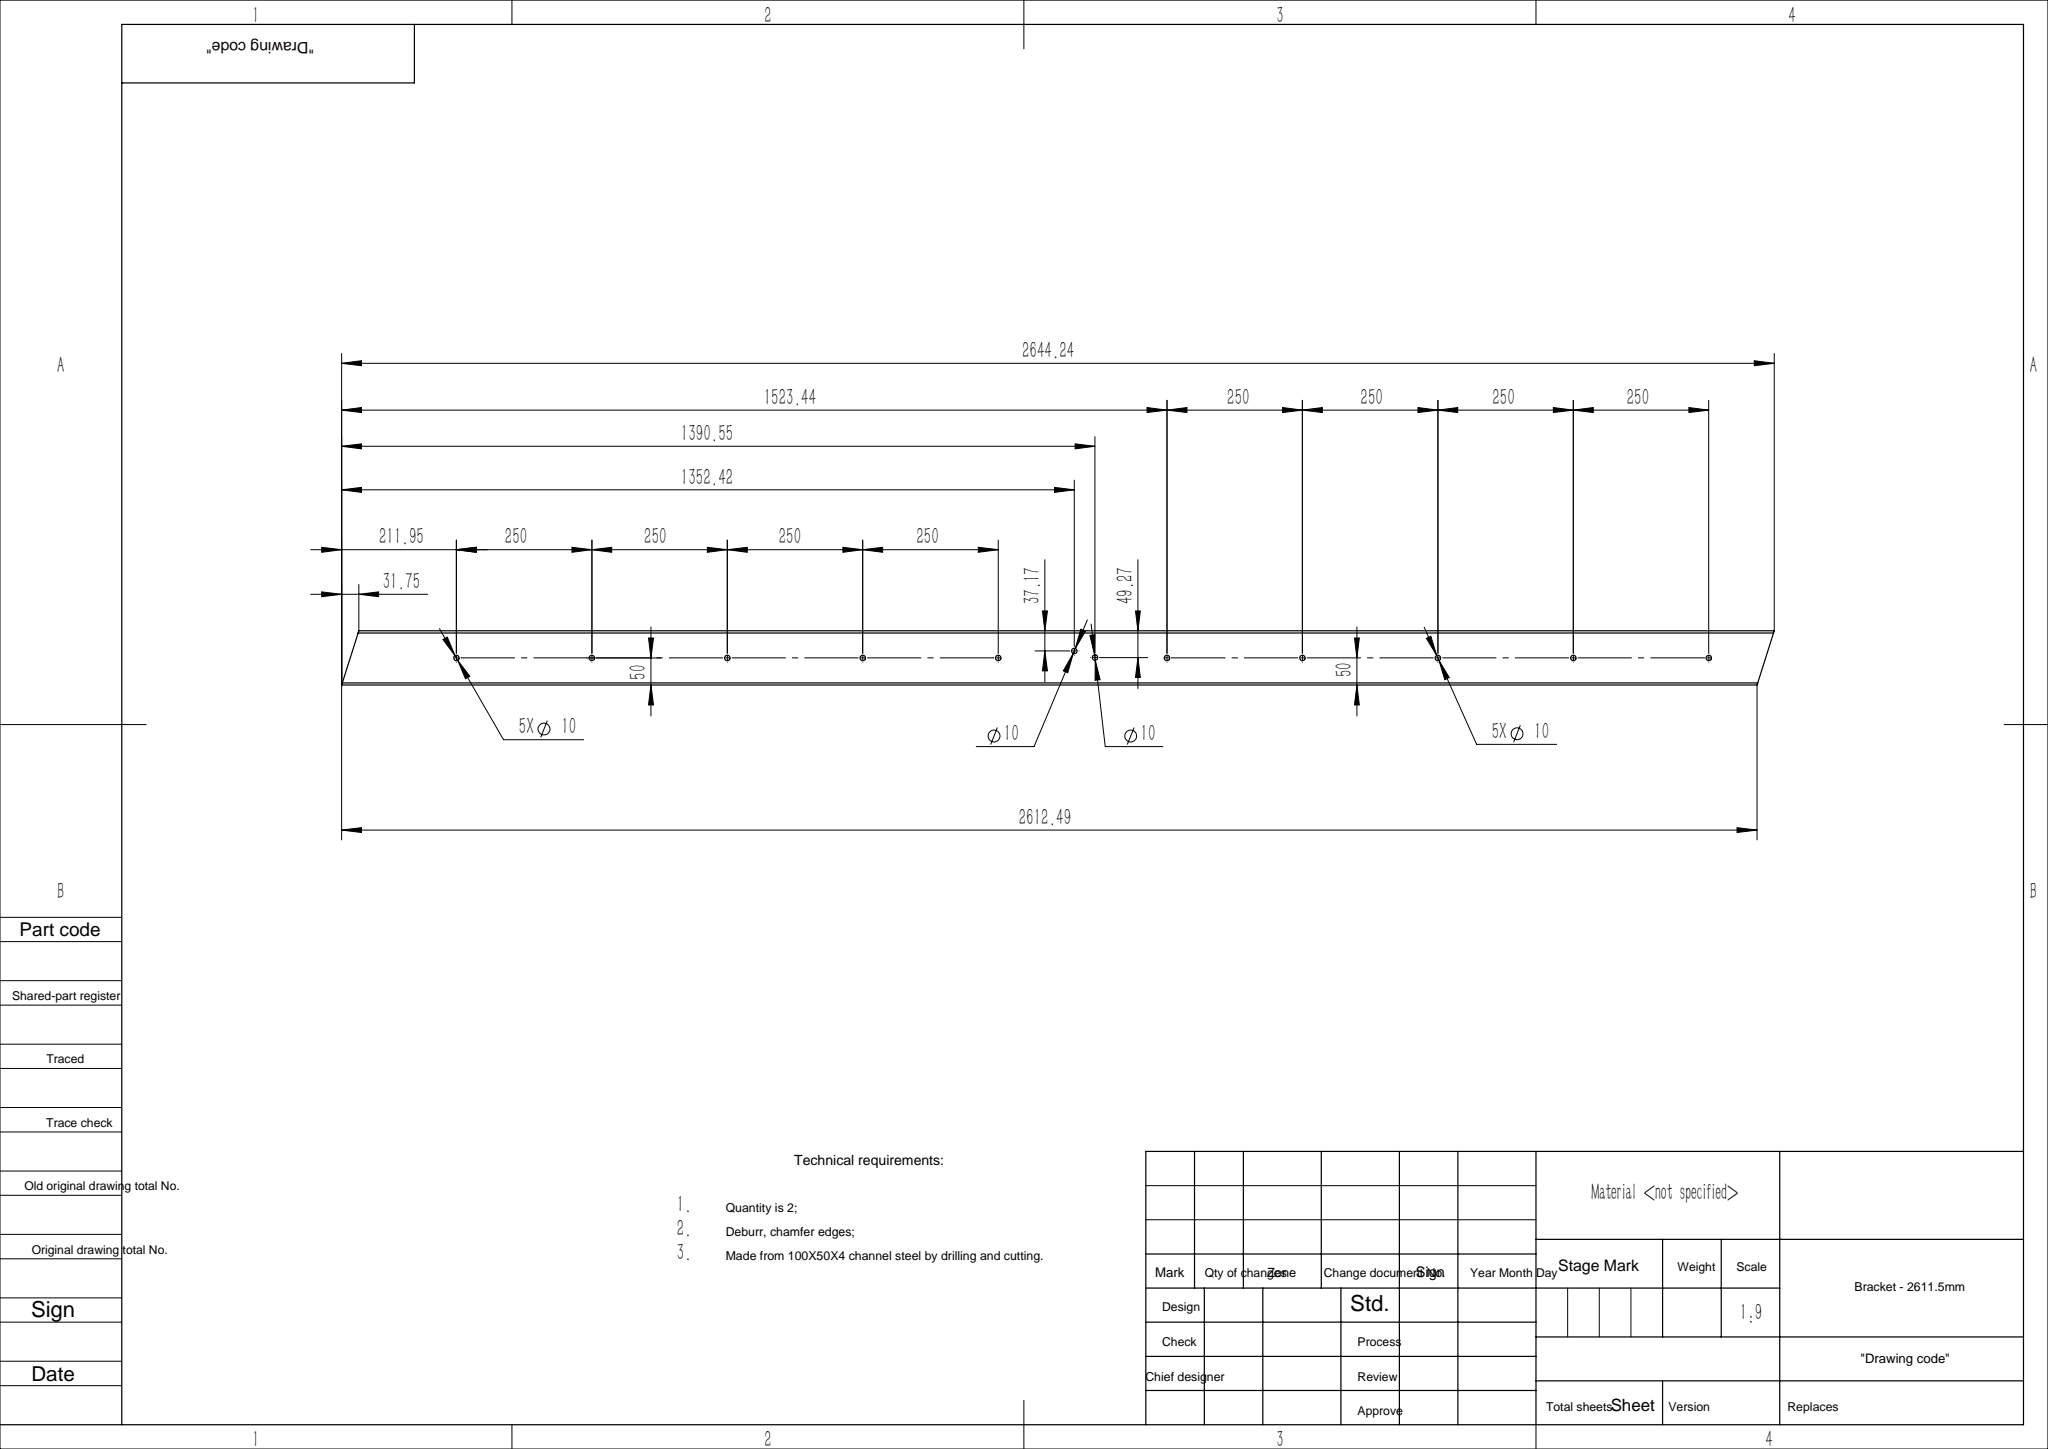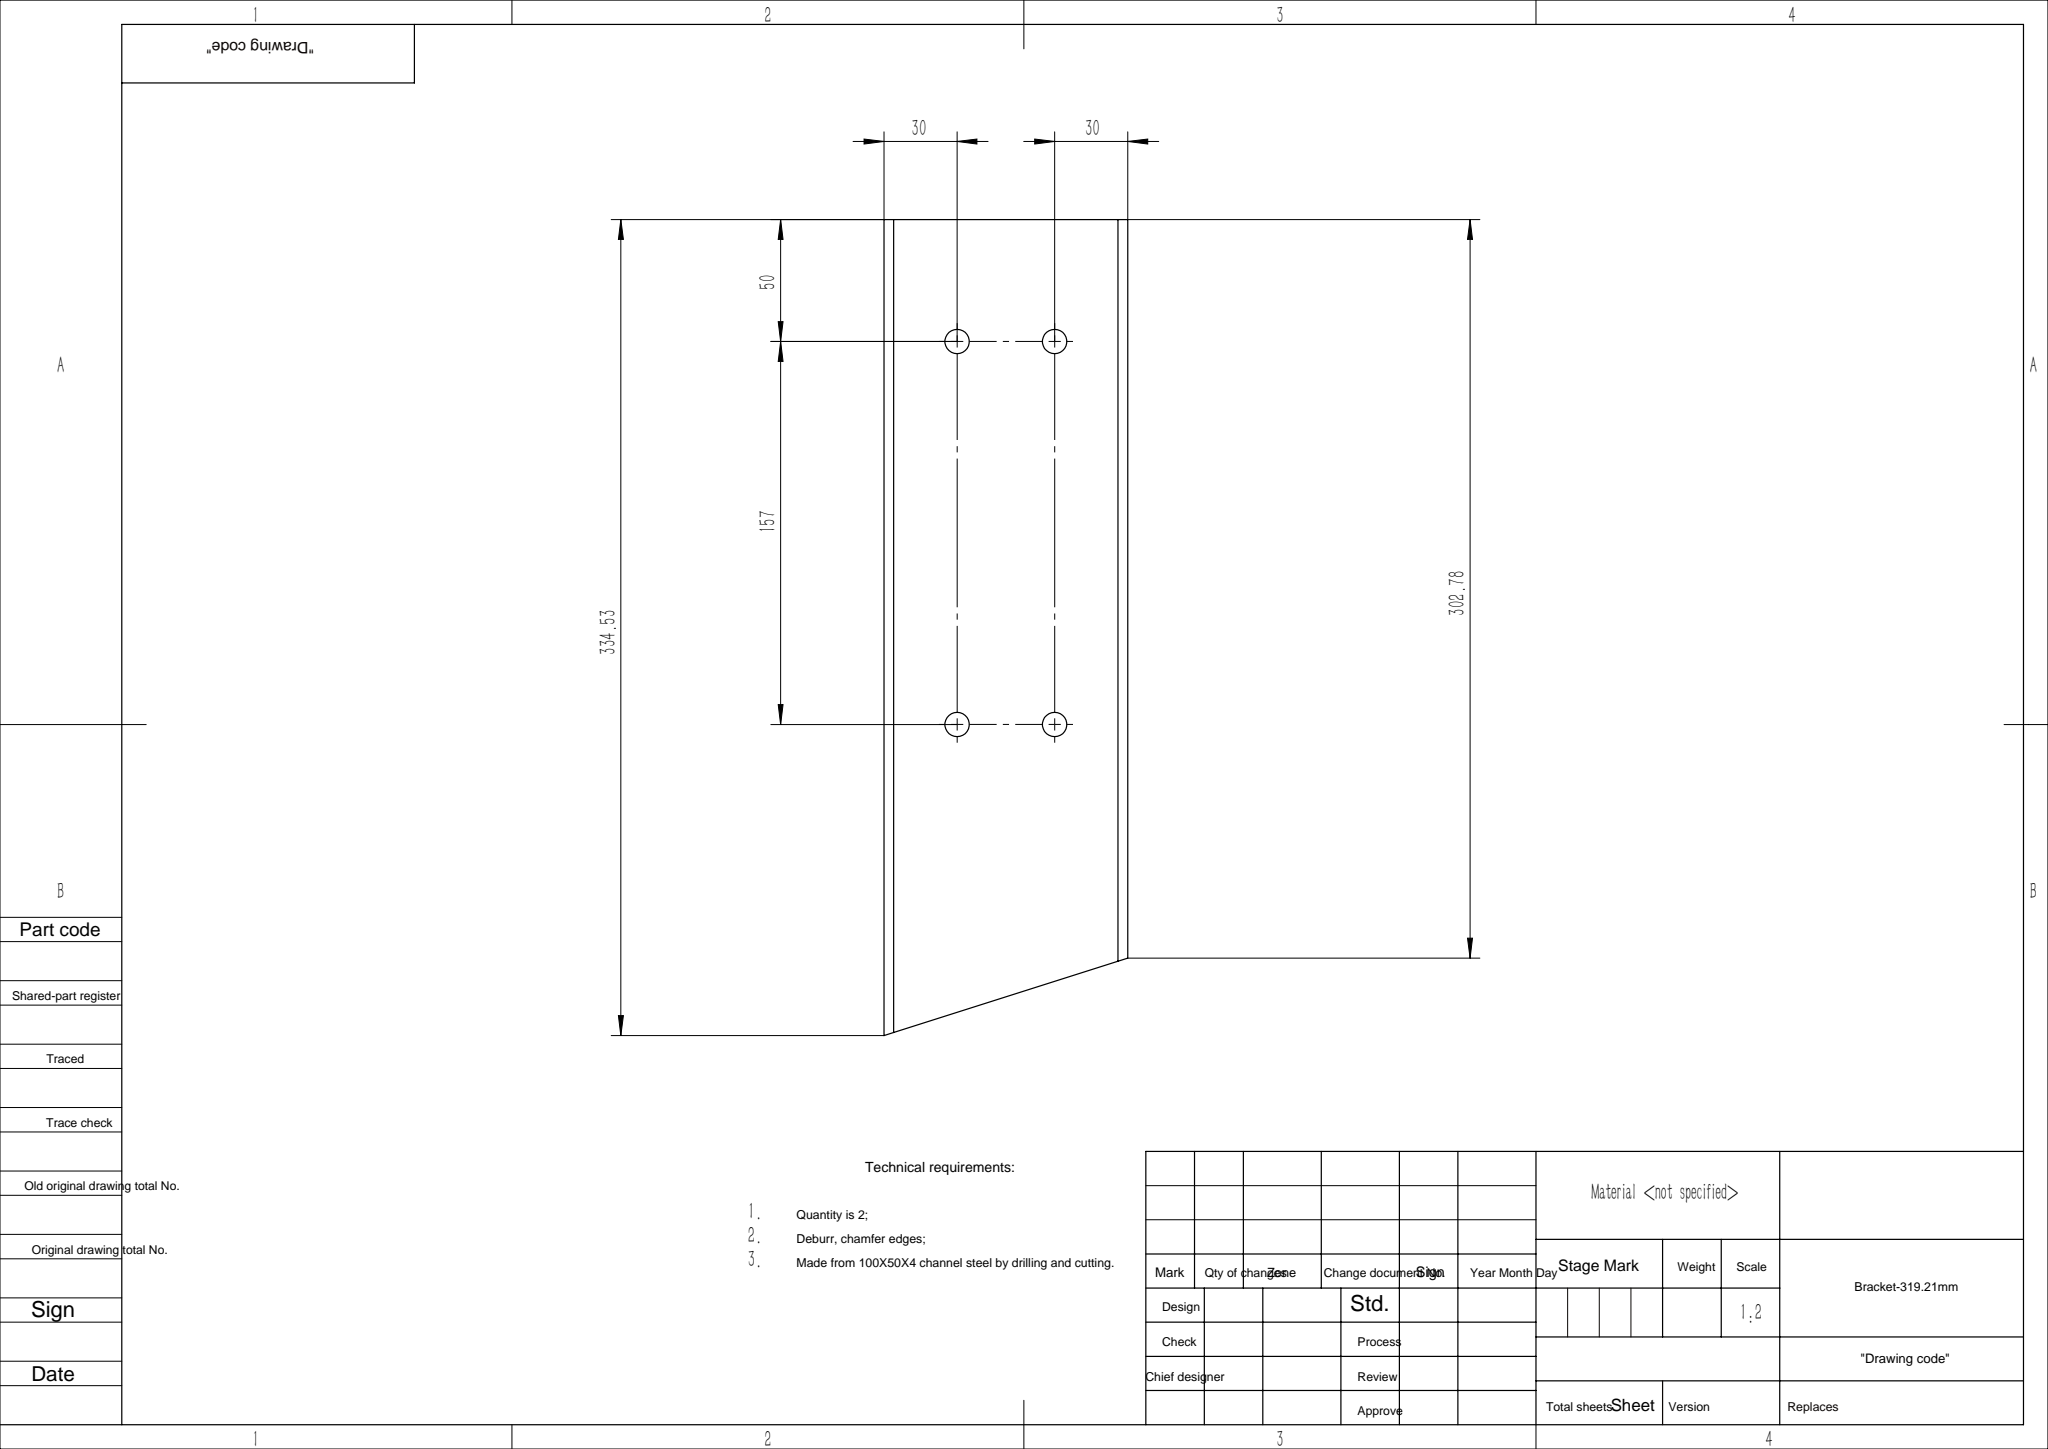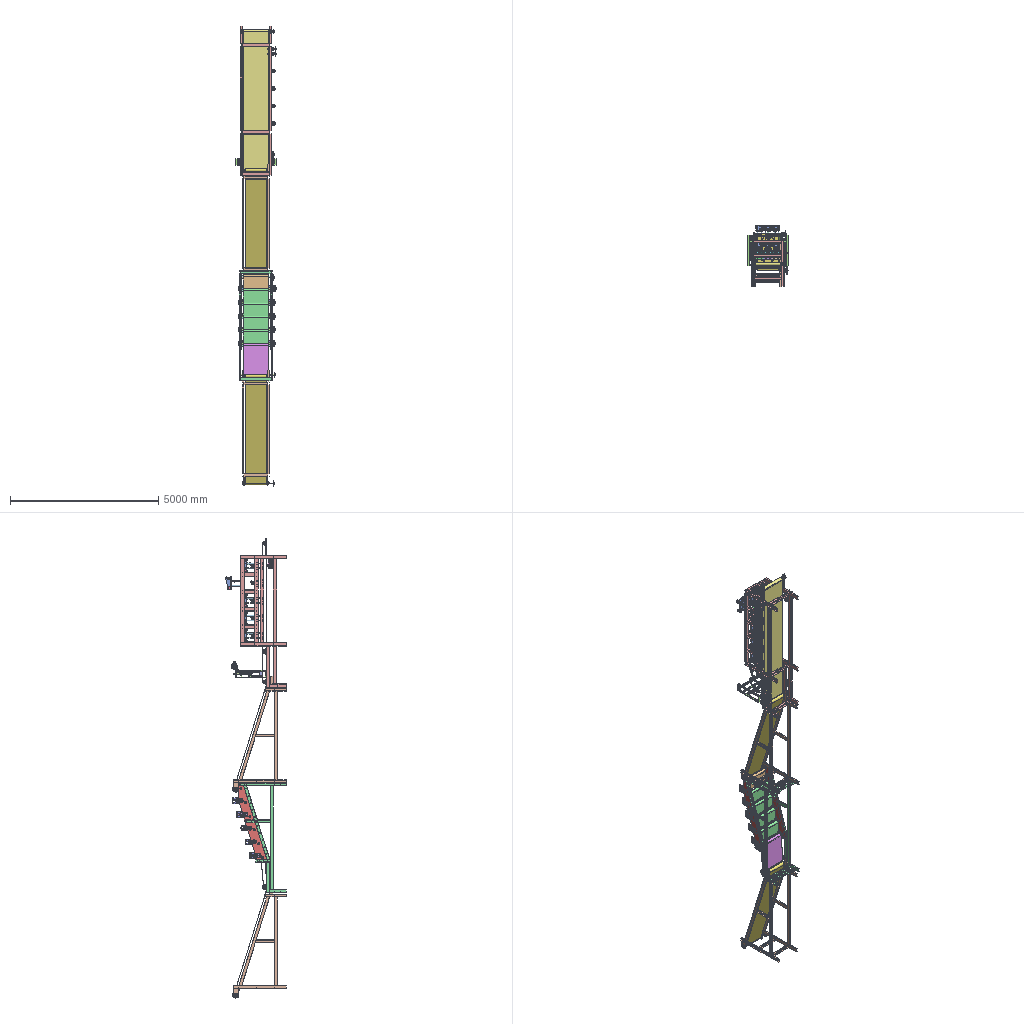Assembly | SolidWorks | 119 different items | 1543 placed | box 1379 x 2047 x 15524 mm
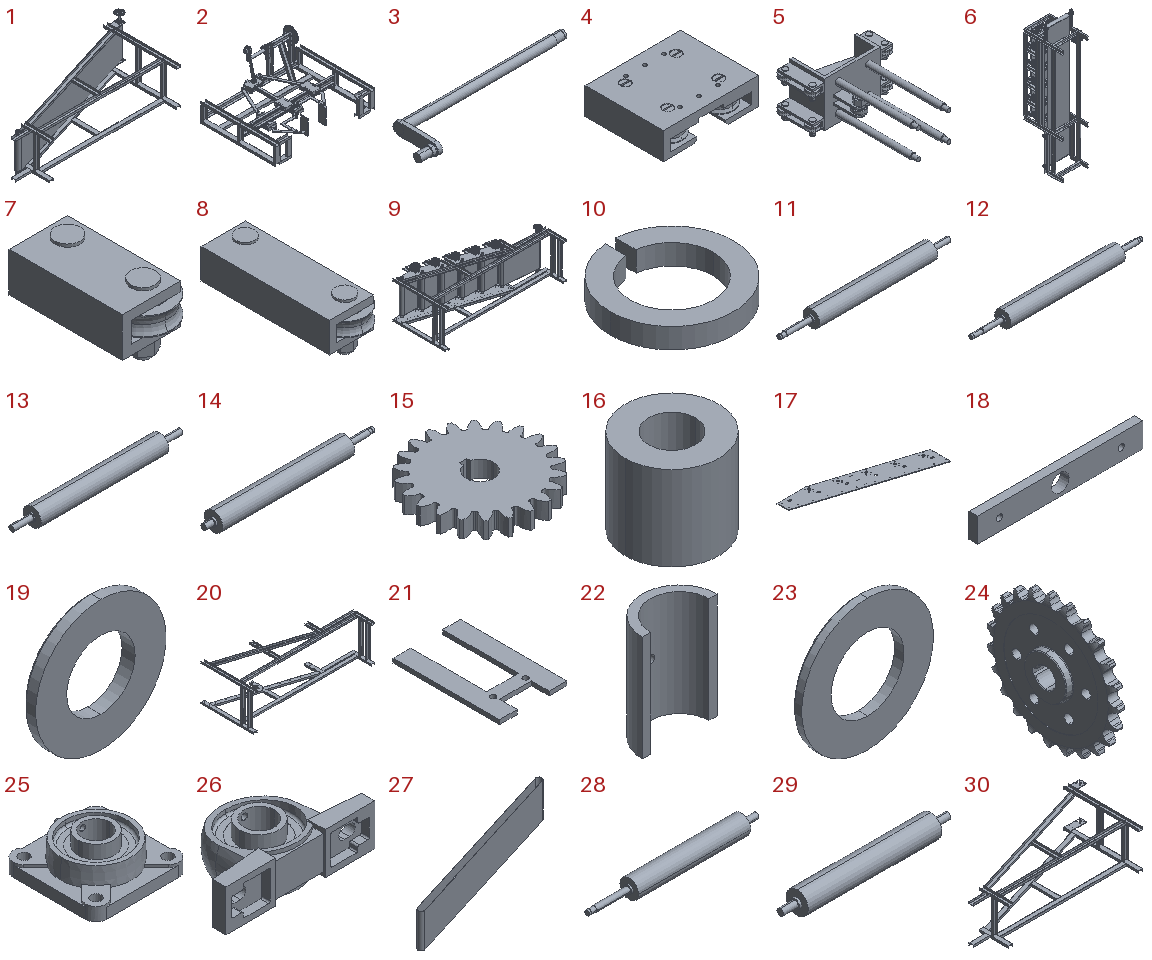Parts list (item | name | quantity | parent item | size | volume | features):
1 | (subassembly) | x2 | - | 3909 x 1808 x 1083 mm | 53217472 mm3 | features MirrorCompFeat 2, ReferencePattern 2
2 | (subassembly) | x1 | - | - | 12242540 mm3 | features LocalLPattern 2, ReferencePattern 2
3 | (subassembly) | x1 | in 2 | 687.7 x 174.987 x 46.865 mm | 737017 mm3 | -
4 | (subassembly) | x5 | in 2 | 135 x 110 x 38 mm | 364943 mm3 | features ReferencePattern 15, LocalLPattern 1
5 | (subassembly) | x15 | in 6 | 430 x 604 x 239 mm | 5255381 mm3 | features ReferencePattern 10, CompositeCurve 1, LocalSketchPattern 1, MirrorCompFeat 1
6 | (subassembly) | x1 | - | - | 264532636 mm3 | features ReferencePattern 140, InContextFeatHolder 10, LocalLPattern 2, LocalSketchPattern 2, MirrorCompFeat 2
7 | (subassembly) | x30 | in 5 | 72 x 140 x 70 mm | 285361 mm3 | -
8 | (subassembly) | x30 | in 5 | 72 x 200 x 70 mm | 372961 mm3 | -
9 | (subassembly) | x1 | - | - | 262282072 mm3 | features ReferencePattern 142, LocalLPattern 5, CompositeCurve 3, MirrorCompFeat 3, AEMSimFeature 1, LocalSketchPattern 1
10 | - | x1 | in 2 | 45.424 x 45.346 x 7.5 mm | 6464 mm3 | features Extrusion 1
11 | - | x1 | in 9 | 1221 x 120 x 120 mm | 9978087 mm3 | features ICE 2, Revolution 1
12 | - | x5 | in 9 | 1261 x 120 x 120 mm | 9997554 mm3 | features ICE 4, Revolution 1
13 | - | x6 | in 9 | 1122 x 120 x 120 mm | 9905091 mm3 | features 3DProfileFeature 1, HoleWzd 1, MirrorPattern 1, Revolution 1
14 | - | x5 | in 9 | 1088 x 120 x 120 mm | 9853270 mm3 | features ICE 2, Revolution 1
15 | - | x10 | in 9 | 133.882 x 132.987 x 18 mm | 197482 mm3 | features ICE 2, CirPattern 1, Extrusion 1, RefAxis 1
16 | - | x20 | in 9 | 30 x 30 x 27 mm | 14314 mm3 | features Extrusion 1
17 | - | x2 | in 9 | 2640 x 1075 x 12 mm | 12600247 mm3 | features Cut 7, LPattern 5, ICE 2, Extrusion 1, SurfCut 1
18 | - | x10 | in 9 | 190 x 10 x 28 mm | 49289 mm3 | features Cut 1, Extrusion 1
19 | - | x1 | in 2 | 20 x 2 x 20 mm | 447.415 mm3 | features Revolution 1
20 | - | x1 | in 9 | 3700 x 1611 x 1120 mm | 19309543 mm3 | features ICE 8, Cut 6, LPattern 6, Extrusion 1, MirrorPattern 1
21 | - | x10 | in 9 | 190 x 300 x 12 mm | 394178 mm3 | features Extrusion 1, HoleWzd 1
22 | - | x12 | in 9 | 46 x 23 x 65 mm | 20833 mm3 | features 3DProfileFeature 1, Extrusion 1, HoleWzd 1
23 | - | x1 | in 2 | 56 x 4 x 56 mm | 6746 mm3 | features Revolution 1
24 | - | x12 | in 9 | 32 x 197.271 x 197.721 mm | 369448 mm3 | features Cut 3, CirPattern 2, Revolution 2, Chamfer 1, Fillet 1, MirrorPattern 1
25 | - | x4 | in 1 | 119 x 119 x 46.4 mm | 215912 mm3 | features Revolution 5, Boss 2, RevCut 2, CirPattern 1, Cut 1, Extrusion 1
26 | - | x4 | in 1 | 172 x 95.2 x 49.4 mm | 226016 mm3 | features Revolution 5, Boss 3, Cut 3, RevCut 2, CirPattern 1, Extrusion 1, SweepCut 1
27 | - | x2 | in 1 | 3723 x 1248 x 720 mm | 17109923 mm3 | features Extrusion 1
28 | - | x2 | in 1 | 1083 x 120 x 120 mm | 8499267 mm3 | features ICE 2, Revolution 1
29 | - | x2 | in 1 | 902 x 120 x 120 mm | 8342146 mm3 | features Revolution 1
30 | - | x2 | in 1 | 3880 x 1780 x 905 mm | 18012747 mm3 | features ICE 8, Cut 3, MirrorPattern 3, Extrusion 1, LPattern 1
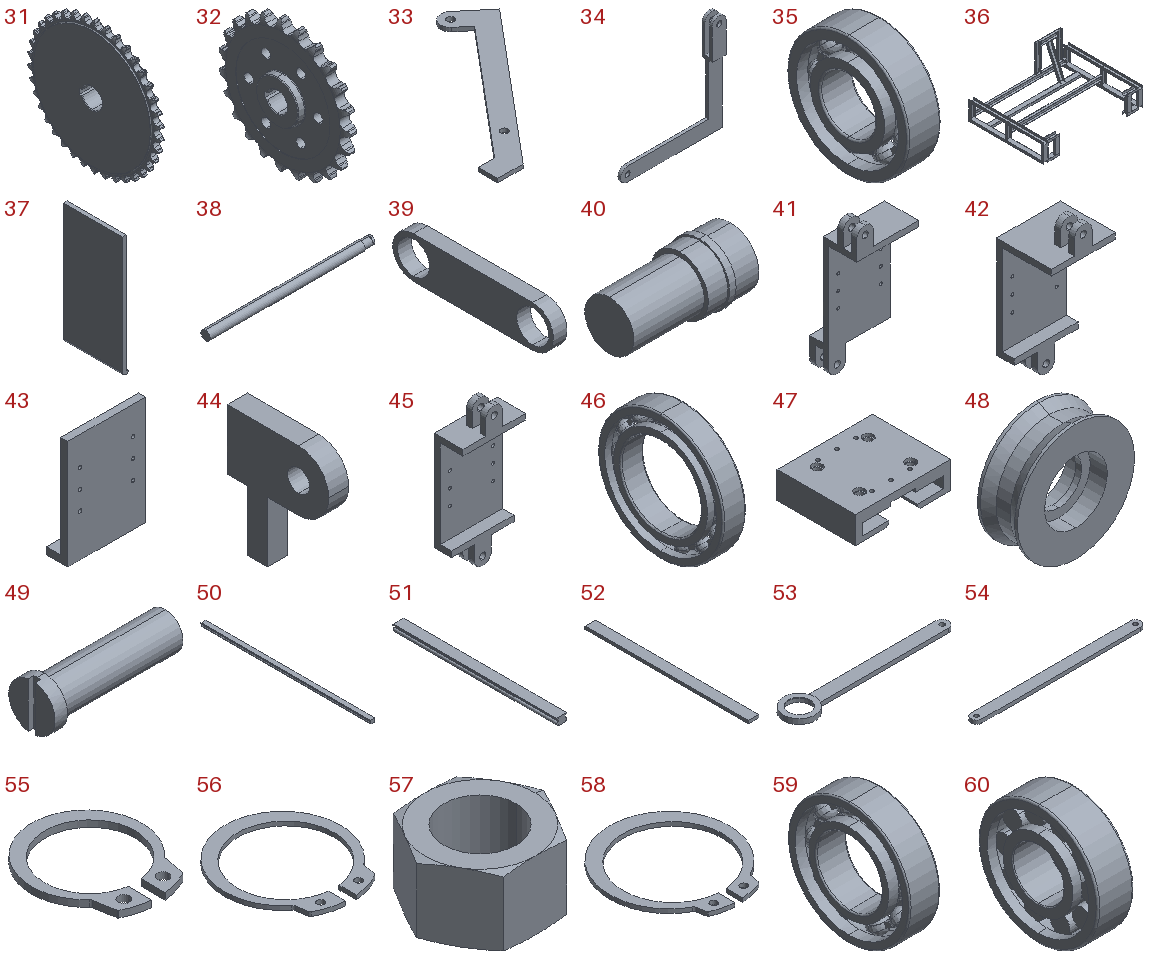31 | - | x1 | in 2 | 32 x 199.417 x 200 mm | 354136 mm3 | features Chamfer 2, Cut 2, Revolution 2, CirPattern 1
32 | - | x2 | in 1 | 32 x 197.271 x 197.721 mm | 369448 mm3 | features Cut 3, CirPattern 2, Revolution 2, Chamfer 1, Fillet 1, MirrorPattern 1
33 | - | x2 | in 2 | 227.962 x 264.071 x 6 mm | 62898 mm3 | features Extrusion 1, Fillet 1
34 | - | x2 | in 2 | 220.41 x 22 x 220.41 mm | 86699 mm3 | features ICE 4, Fillet 2, Extrusion 1
35 | - | x40 | in 4 | 6 x 22 x 22 mm | 1184 mm3 | features Revolution 5, CirPattern 2, RevCut 2
36 | - | x1 | in 2 | 1372 x 1032 x 491.47 mm | 3956578 mm3 | features ICE 10, Extrusion 1, MirrorPattern 1, RefAxis 1, RefPoint 1
37 | - | x2 | in 2 | 9.928 x 100 x 205.732 mm | 123626 mm3 | features Extrusion 1, Fillet 1
38 | - | x1 | in 3 | 628.7 x 35 x 35 mm | 593601 mm3 | features ICE 2, Cut 1, Extrusion 1
39 | - | x1 | in 3 | 15 x 175 x 45 mm | 82743 mm3 | features ICE 2, Extrusion 1
40 | - | x1 | in 3 | 74 x 37 x 37 mm | 60673 mm3 | features ICE 2, Extrusion 1
41 | - | x1 | in 2 | 110 x 100 x 255 mm | 333226 mm3 | features ICE 7, Fillet 3, LPattern 3, Extrusion 1, HoleWzd 1
42 | - | x1 | in 2 | 110 x 94 x 255 mm | 346058 mm3 | features ICE 6, Fillet 2, LPattern 2, Extrusion 1, HoleWzd 1
43 | - | x2 | in 2 | 110 x 30 x 155 mm | 191322 mm3 | features ICE 2, Extrusion 1, HoleWzd 1
44 | - | x4 | in 2 | 10 x 50.5 x 60 mm | 16234 mm3 | features Extrusion 1, Fillet 1
45 | - | x1 | in 2 | 110 x 50 x 255 mm | 297658 mm3 | features ICE 6, Fillet 2, LPattern 2, Extrusion 1, HoleWzd 1
46 | - | x1 | in 2 | 10 x 55 x 55 mm | 9427 mm3 | features Revolution 5, CirPattern 2, RevCut 2
47 | - | x5 | in 4 | 135 x 110 x 38 mm | 295400 mm3 | features ICE 4, LPattern 2, Chamfer 1, Extrusion 1, HoleWzd 1
48 | - | x20 | in 4 | 41 x 14 x 41 mm | 11422 mm3 | features Revolution 1
49 | - | x20 | in 4 | 37.5 x 13 x 13 mm | 3096 mm3 | features Chamfer 1, Cut 1, ICE 1, Revolution 1
50 | - | x2 | in 2 | 36 x 1252 x 25 mm | 935920 mm3 | features Extrusion 1
51 | - | x1 | in 2 | 36 x 563 x 25 mm | 420865 mm3 | features Extrusion 1
52 | - | x1 | in 2 | 36 x 563 x 10 mm | 202680 mm3 | features Extrusion 1
53 | - | x1 | in 2 | 392.5 x 75 x 12 mm | 118812 mm3 | features Extrusion 1, Fillet 1, ICE 1
54 | - | x2 | in 2 | 474.13 x 30 x 10 mm | 138407 mm3 | features Extrusion 1, Fillet 1
55 | - | x2 | in 6 | 16.8 x 19.352 x 1 mm | 89.212 mm3 | features Extrusion 1
56 | - | x3 | in 6 | 33.5 x 36.571 x 1.2 mm | 375.293 mm3 | features Extrusion 1
57 | - | x1 | in 2 | 17.59 x 15.233 x 9.5 mm | 1159 mm3 | features Cut 2, Chamfer 1, Extrusion 1
58 | - | x5 | in 6 | 44 x 47.504 x 1.5 mm | 776.12 mm3 | features Extrusion 1
59 | - | x2 | in 6 | 7 x 28 x 28 mm | 1855 mm3 | features Revolution 5, CirPattern 2, RevCut 2
60 | - | x120 | in 7, 8 | 12 x 40 x 40 mm | 7964 mm3 | features Revolution 3, CirPattern 1
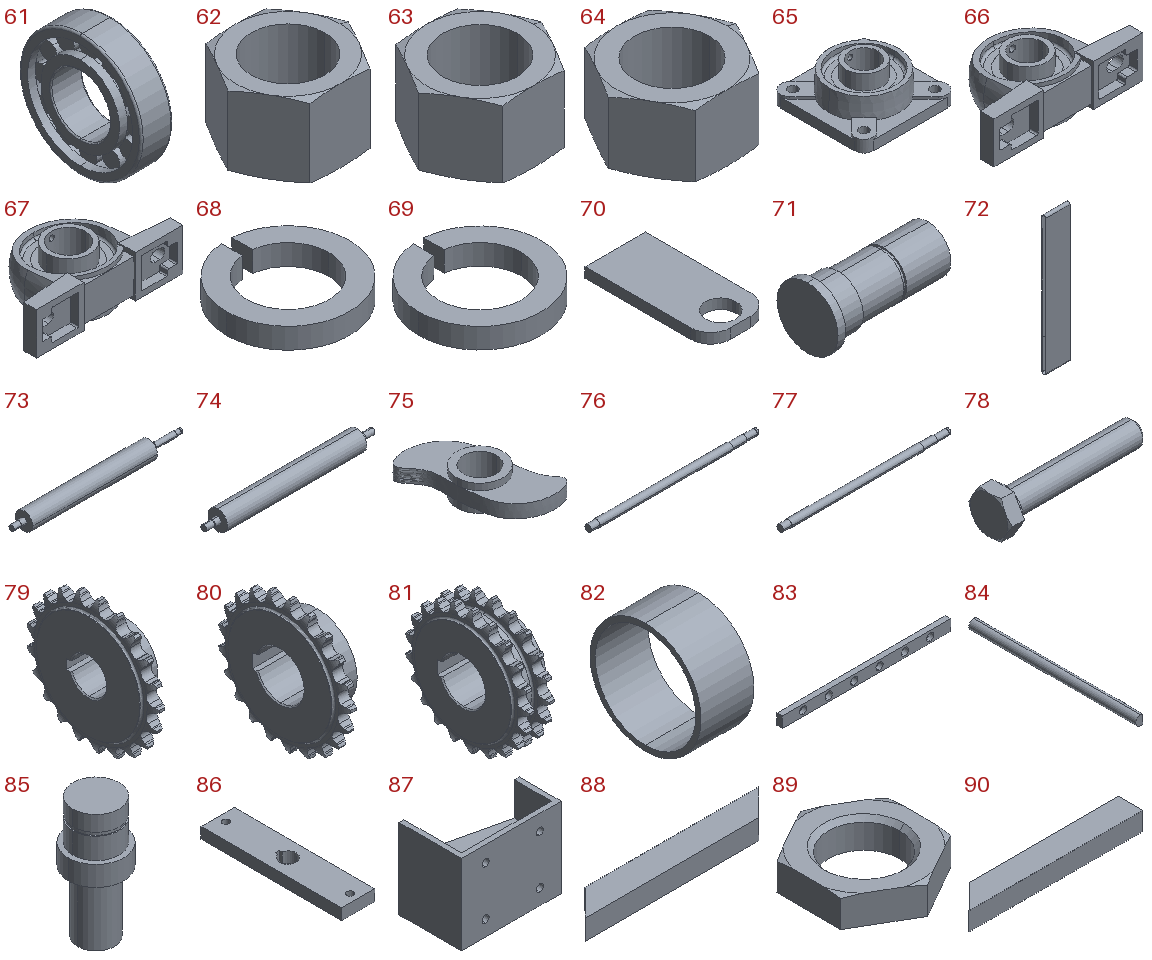61 | - | x15 | in 5 | 16 x 62 x 62 mm | 24506 mm3 | features Revolution 3, CirPattern 1
62 | - | x120 | in 7, 8 | 26.17 x 22.664 x 15.9 mm | 3864 mm3 | features Cut 2, Chamfer 1, Extrusion 1
63 | - | x60 | in 5 | 32.95 x 28.536 x 19 mm | 7406 mm3 | features Cut 2, Chamfer 1, Extrusion 1
64 | - | x16 | in 2, 5 | 50.85 x 44.037 x 26.4 mm | 25591 mm3 | features Cut 2, Chamfer 1, Extrusion 1
65 | - | x4 | in 6 | 132 x 132 x 54.2 mm | 283670 mm3 | features Revolution 5, Boss 2, RevCut 2, CirPattern 1, Cut 1, Extrusion 1
66 | - | x8 | in 6, 9 | 172 x 95.2 x 49.4 mm | 226016 mm3 | features Revolution 5, Boss 3, Cut 3, RevCut 2, CirPattern 1, Extrusion 1, SweepCut 1
67 | - | x10 | in 6 | 192 x 109.26 x 57.7 mm | 325888 mm3 | features Revolution 5, Boss 3, Cut 3, RevCut 2, CirPattern 1, Extrusion 1, SweepCut 1
68 | - | x120 | in 7, 8 | 24.356 x 24.313 x 4.1 mm | 1031 mm3 | features Extrusion 1
69 | - | x60 | in 5 | 30.149 x 30.097 x 5 mm | 1905 mm3 | features Extrusion 1
70 | - | x30 | in 5 | 60 x 125 x 10 mm | 66120 mm3 | features Extrusion 1, Fillet 1
71 | - | x15 | in 5 | 79 x 40 x 40 mm | 60635 mm3 | features ICE 1, Revolution 1
72 | - | x1 | in 6 | 850 x 135 x 4803 mm | 41389503 mm3 | features Extrusion 1
73 | - | x1 | in 6 | 1154 x 120 x 120 mm | 9914503 mm3 | features ICE 2, Revolution 1
74 | - | x2 | in 6 | 1027 x 120 x 120 mm | 9804184 mm3 | features Revolution 1
75 | - | x15 | in 6 | 114.053 x 172.33 x 40 mm | 212342 mm3 | features BaseBody 1
76 | - | x1 | in 6 | 1162 x 50 x 50 mm | 2157809 mm3 | features ICE 2, Revolution 1
77 | - | x4 | in 6 | 1172 x 50 x 50 mm | 2169811 mm3 | features ICE 2, Revolution 1
78 | - | x1 | in 2 | 61.4 x 18.475 x 16 mm | 5702 mm3 | features RevCut 4, Chamfer 1, Extrusion 1, Fillet 1, LPattern 1, Revolution 1
79 | - | x3 | in 6 | 32 x 112.513 x 112.819 mm | 118760 mm3 | features Chamfer 2, Cut 2, Revolution 2, CirPattern 1
80 | - | x1 | in 6 | 32 x 112.513 x 112.819 mm | 125263 mm3 | features Chamfer 2, Cut 2, Revolution 2, CirPattern 1
81 | - | x9 | in 6 | 42 x 112.513 x 112.819 mm | 211339 mm3 | features Revolution 3, Chamfer 2, Cut 2, CirPattern 1, LPattern 1
82 | - | x1 | in 6 | 20 x 42 x 42 mm | 5027 mm3 | features Extrusion 1
83 | - | x10 | in 6 | 930 x 30 x 60 mm | 1426600 mm3 | features Extrusion 1, LPattern 1, RevCut 1
84 | - | x60 | in 6 | 30 x 531 x 30 mm | 358759 mm3 | features Extrusion 1, ICE 1, MirrorPattern 1
85 | - | x2 | in 6 | 18 x 18 x 39.5 mm | 6196 mm3 | features ICE 1, Revolution 1
86 | - | x1 | in 6 | 60 x 256 x 20 mm | 287870 mm3 | features ICE 2, Extrusion 1
87 | - | x15 | in 5 | 286 x 180 x 230 mm | 2480573 mm3 | features ICE 3, Extrusion 1, LPattern 1
88 | - | x5 | in 6 | 300 x 40 x 30 mm | 293150 mm3 | features ICE 5, Extrusion 1
89 | - | x20 | in 4 | 15.424 x 17.77 x 4 mm | 499.386 mm3 | features Cut 3, Chamfer 1, Extrusion 1
90 | - | x5 | in 6 | 285 x 40 x 30 mm | 299150 mm3 | features ICE 3, Extrusion 1
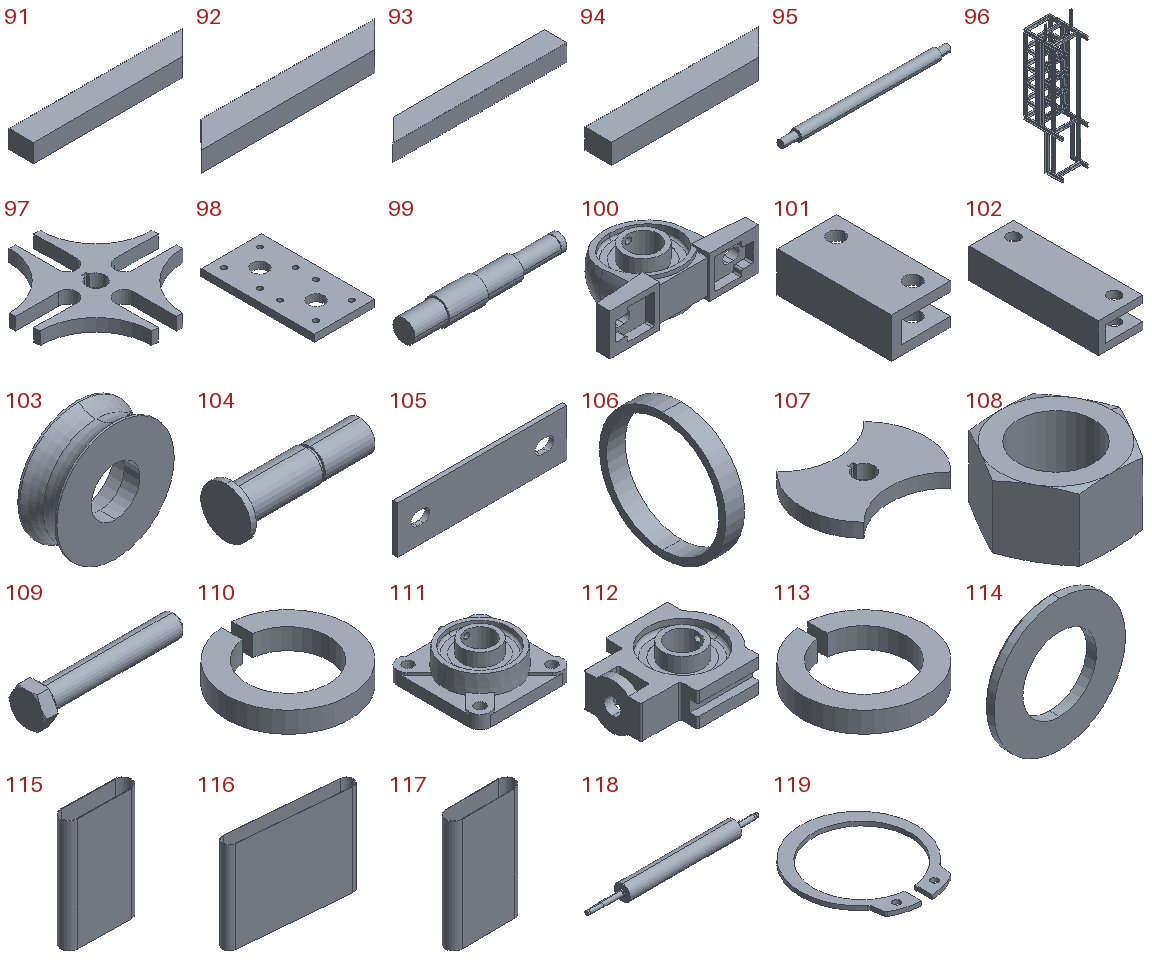91 | - | x5 | in 6 | 285 x 40 x 30 mm | 299150 mm3 | features ICE 3, Extrusion 1
92 | - | x5 | in 6 | 300 x 40 x 30 mm | 293150 mm3 | features ICE 5, Extrusion 1
93 | - | x5 | in 6 | 310 x 40 x 30 mm | 329150 mm3 | features ICE 3, Extrusion 1
94 | - | x5 | in 6 | 260 x 40 x 30 mm | 269150 mm3 | features ICE 3, Extrusion 1
95 | - | x60 | in 5 | 457 x 30 x 30 mm | 294248 mm3 | features ICE 1, Revolution 1
96 | - | x1 | in 6 | 1050 x 1536 x 5045 mm | 54295984 mm3 | features ICE 10, LPattern 7, SketchPattern 2, CombineBodies 1, Extrusion 1
97 | - | x1 | in 6 | 226 x 226 x 20 mm | 323125 mm3 | features Extrusion 1, ICE 1
98 | - | x2 | in 6 | 172 x 322 x 20 mm | 1019433 mm3 | features Cut 1, Extrusion 1
99 | - | x2 | in 6 | 280.7 x 46 x 46 mm | 333070 mm3 | features ICE 2, Revolution 1
100 | - | x2 | in 2 | 172 x 95.2 x 49.4 mm | 226016 mm3 | features Revolution 5, Boss 3, Cut 3, RevCut 2, CirPattern 1, Extrusion 1, SweepCut 1
101 | - | x30 | in 7 | 62 x 120 x 42 mm | 165906 mm3 | features Extrusion 1, ICE 1
102 | - | x30 | in 8 | 62 x 180 x 42 mm | 253506 mm3 | features Extrusion 1, ICE 1
103 | - | x120 | in 7, 8 | 60 x 20 x 60 mm | 30888 mm3 | features ICE 2, Extrusion 1, RevCut 1
104 | - | x120 | in 7, 8 | 70 x 26 x 26 mm | 15980 mm3 | features ICE 2, Revolution 1
105 | - | x2 | in 6 | 172 x 5 x 48 mm | 39173 mm3 | features Cut 1, Extrusion 1
106 | - | x15 | in 5 | 5 x 34 x 34 mm | 958.029 mm3 | features Extrusion 1
107 | - | x1 | in 6 | 176 x 124.451 x 20 mm | 294954 mm3 | features Extrusion 1, ICE 1
108 | - | x12 | in 9 | 60.79 x 52.646 x 31.9 mm | 43950 mm3 | features Cut 2, Chamfer 1, Extrusion 1
109 | - | x10 | in 9 | 121.5 x 31.177 x 27 mm | 35083 mm3 | features RevCut 4, Chamfer 1, Extrusion 1, Fillet 1, LPattern 1, Revolution 1
110 | - | x1 | in 2 | 15.372 x 15.344 x 2.6 mm | 261.313 mm3 | features Extrusion 1
111 | - | x10 | in 9 | 119 x 119 x 46.4 mm | 215912 mm3 | features Revolution 5, Boss 2, RevCut 2, CirPattern 1, Cut 1, Extrusion 1
112 | - | x10 | in 9 | 132 x 107 x 53 mm | 274661 mm3 | features Revolution 6, RevCut 3, Cut 1, Extrusion 1
113 | - | x12 | in 9 | 53.421 x 53.336 x 9 mm | 10431 mm3 | features Extrusion 1
114 | - | x12 | in 9 | 66 x 5 x 66 mm | 11570 mm3 | features Revolution 1
115 | - | x1 | in 9 | 525.939 x 132.981 x 850 mm | 3025361 mm3 | features Extrusion 1
116 | - | x1 | in 9 | 1122 x 213.156 x 850 mm | 6085361 mm3 | features Extrusion 1
117 | - | x4 | in 9 | 525.939 x 129.019 x 850 mm | 3025108 mm3 | features Extrusion 1
118 | - | x1 | in 9 | 1293 x 120 x 120 mm | 10019195 mm3 | features ICE 4, Revolution 1
119 | - | x1 | in 2 | 33.5 x 36.571 x 1.2 mm | 375.293 mm3 | features Extrusion 1
Mates (type | each side: item.copy, entity, surface, feature), first 226 of 386 lines:
In the top assembly
Width | 36.1 face plane Boss-Extrude 2 | 36.1 face plane Boss-Extrude 2 | 96.1 face plane Boss-Extrude 8 | 96.1 face plane Boss-Extrude 8
Coincident | 36.1 face plane Boss-Extrude 3 | 96.1 face plane Boss-Extrude 8
DistanceDim | 36.1 face plane Boss-Extrude 3 | 66.1 face plane Boss-Extrude 1
Coincident | 96.1 face plane Boss-Extrude 9 | 30.1 face plane Boss-Extrude 1
Width | 30.1 face plane Boss-Extrude 1 | 30.1 face plane Boss-Extrude 1 | 96.1 face plane Boss-Extrude 9 | 96.1 face plane Boss-Extrude 9
Coincident | 30.1 face plane Boss-Extrude 3 | 20.1 face plane Boss-Extrude 1 | 2 times
Width | 20.1 face plane Boss-Extrude 1 | 20.1 face plane Boss-Extrude 1 | 30.1 face plane Boss-Extrude 3 | 30.1 face plane Boss-Extrude 3
Coincident | 20.1 face plane Boss-Extrude 3 | 30.2 face plane Boss-Extrude 1
Width | 30.2 face plane Boss-Extrude 1 | 30.2 face plane Boss-Extrude 1 | 20.1 face plane Boss-Extrude 3 | 20.1 face plane Boss-Extrude 3
DistanceDim | 20.1 face plane Boss-Extrude 3 | 30.2 face plane Boss-Extrude 1
DistanceDim | 96.1 face plane Boss-Extrude 8 | 30.1 face plane Boss-Extrude 1
In subassembly 1
Coincident | 30.3 face plane Boss-Extrude 6 | 25.1 face plane Base-Extrude
DistanceDim | 25.1 face plane Base-Extrude | 30.3 face plane Boss-Extrude 6 | 2 times
Concentric | 30.3 face cylinder Cut-Extrude 1 | 28.1 face cylinder Revolve 1
Symmetric | 28.1 face plane Revolve 1 | 28.1 face plane Revolve 1 | 1.1 plane
Coincident | 28.1 face plane Revolve 1 | 32.1 face plane Revolve 2
Concentric | 28.1 face cylinder Revolve 1 | 32.1 face cylinder Revolve 1
Symmetric | 29.1 face plane Revolve 1 | 29.1 face plane Revolve 1 | 1.1 plane
Coincident | 30.3 face plane Boss-Extrude 8 | 26.1 face plane Boss-Extrude 1
Concentric | 29.1 face cylinder Revolve 1 | 26.1 face cylinder Boss-Revolve 5
Coincident | 30.3 face plane Boss-Extrude 1 | 26.1 face plane Boss-Extrude 1
DistanceDim | 26.1 face plane Boss-Extrude 1 | 30.3 face plane Boss-Extrude 1
In subassembly 6
DistanceDim | 87.1 face plane Boss-Extrude 1 | 96.2 face plane Boss-Extrude 1
Parallel | 96.2 face plane Boss-Extrude 1 | 87.1 face plane Boss-Extrude 1
Coincident | 96.2 face plane LPattern 7 | 84.1 face plane Cut-Extrude 1
Coincident | 96.2 face plane Boss-Extrude 1 | 84.1 face plane Boss-Extrude 1
Tangent | 103.1 face torus Cut-Revolve 1 | 6.1 plane
Concentric | 95.1 face cylinder Revolve 1 | 90.1 face cylinder Cut-Extrude 2
Concentric | 95.2 face cylinder Revolve 1 | 90.1 face cylinder Cut-Extrude 2
Coincident | 95.1 face plane Revolve 1 | 90.1 face plane Boss-Extrude 1
Concentric | 95.3 face cylinder Revolve 1 | 88.1 face cylinder Cut-Extrude 2
Coincident | 95.3 face plane Revolve 1 | 88.1 face plane Boss-Extrude 1
Concentric | 95.4 face cylinder Revolve 1 | 88.1 face cylinder Cut-Extrude 2
Concentric | 95.5 face cylinder Revolve 1 | 91.1 face cylinder Cut-Extrude 2
Concentric | 95.6 face cylinder Revolve 1 | 91.1 face cylinder Cut-Extrude 2
Coincident | 95.6 face plane Revolve 1 | 91.1 face plane Boss-Extrude 1
Concentric | 95.7 face cylinder Revolve 1 | 93.1 face cylinder Cut-Extrude 2
Concentric | 95.8 face cylinder Revolve 1 | 93.1 face cylinder Cut-Extrude 2
Coincident | 95.7 face plane Revolve 1 | 93.1 face plane Boss-Extrude 1
Concentric | 95.9 face cylinder Revolve 1 | 92.1 face cylinder Cut-Extrude 2
Coincident | 95.9 face plane Revolve 1 | 92.1 face plane Boss-Extrude 1
Concentric | 95.10 face cylinder Revolve 1 | 92.1 face cylinder Cut-Extrude 2
Concentric | 95.11 face cylinder Revolve 1 | 94.1 face cylinder Cut-Extrude 2
Concentric | 95.12 face cylinder Revolve 1 | 94.1 face cylinder Cut-Extrude 2
Coincident | 95.11 face plane Revolve 1 | 94.1 face plane Boss-Extrude 1
Coincident | 96.2 face plane LPattern 6 | 67.1 face plane Boss-Extrude 1
Coincident | 96.2 face plane LPattern 6 | 67.2 face plane Boss-Extrude 1
Coincident | 96.2 face plane Boss-Extrude 1 | 67.1 face plane Boss-Extrude 1
Coincident | 96.2 face plane Boss-Extrude 1 | 67.2 face plane Boss-Extrude 1
Concentric | 67.1 face cylinder Boss-Revolve 5 | 77.1 face cylinder Revolve 1
Coincident | 67.2 face plane Boss-Revolve 5 | 77.1 face plane Revolve 1
Concentric | 77.1 face cylinder Revolve 1 | 75.1 face cylinder  Import 1
Width | 75.1 face plane  Import 1 | 75.1 face plane  Import 1 | 87.1 face plane Boss-Extrude 1 | 87.1 face plane Boss-Extrude 1
Coincident | 96.2 face plane Boss-Extrude 4 | 66.2 face plane Boss-Extrude 1
Coincident | 96.2 face plane Boss-Extrude 1 | 66.2 face plane Boss-Extrude 1
DistanceDim | 66.2 face plane Boss-Extrude 1 | 96.2 face plane Boss-Extrude 4
Coincident | 96.2 face plane Boss-Extrude 4 | 66.3 face plane Boss-Extrude 1
Coincident | 96.2 face plane Boss-Extrude 1 | 66.3 face plane Boss-Extrude 1
Coincident | 66.2 face plane Boss-Extrude 1 | 66.3 face plane Boss-Extrude 1
Concentric | 66.2 face cylinder Boss-Revolve 5 | 73.1 face cylinder Revolve 1
Coincident | 66.3 face plane Boss-Revolve 5 | 73.1 face plane Revolve 1
Coincident | 96.2 face plane Boss-Extrude 8 | 66.4 face plane Boss-Extrude 1
Coincident | 96.2 face plane Boss-Extrude 1 | 66.4 face plane Boss-Extrude 1
DistanceDim | 66.4 face plane Boss-Extrude 1 | 96.2 face plane Boss-Extrude 8
Coincident | 96.2 face plane Boss-Extrude 8 | 66.5 face plane Boss-Extrude 1
Coincident | 96.2 face plane Boss-Extrude 1 | 66.5 face plane Boss-Extrude 1
Coincident | 66.4 face plane Boss-Extrude 1 | 66.5 face plane Boss-Extrude 1
Concentric | 66.5 face cylinder Boss-Revolve 5 | 74.1 face cylinder Revolve 1
Coincident | 66.5 face plane Boss-Revolve 5 | 74.1 face plane Revolve 1
Coincident | 96.2 face plane Boss-Extrude 8 | 105.1 face plane Boss-Extrude 1
Coincident | 96.2 face plane Boss-Extrude 1 | 105.1 face plane Boss-Extrude 1
DistanceDim | 105.1 face plane Boss-Extrude 1 | 96.2 face plane LPattern 1
Coincident | 105.1 face plane Boss-Extrude 1 | 66.6 face plane Base-Extrude
Coincident | 96.2 face plane Boss-Extrude 1 | 66.6 face plane Boss-Extrude 1
Coincident | 105.1 face plane Boss-Extrude 1 | 66.6 face plane Boss-Extrude 1
Coincident | 96.2 face plane Boss-Extrude 1 | 105.2 face plane Boss-Extrude 1
Coincident | 96.2 face plane Boss-Extrude 8 | 105.2 face plane Boss-Extrude 1
Coincident | 105.1 face plane Boss-Extrude 1 | 105.2 face plane Boss-Extrude 1
Coincident | 105.2 face plane Boss-Extrude 1 | 66.7 face plane Boss-Extrude 1
Coincident | 96.2 face plane Boss-Extrude 1 | 66.7 face plane Boss-Extrude 1
Coincident | 66.6 face plane Boss-Extrude 1 | 66.7 face plane Boss-Extrude 1
Concentric | 66.6 face cylinder Boss-Revolve 5 | 74.2 face cylinder Revolve 1
Coincident | 66.7 face plane Boss-Revolve 5 | 74.2 face plane Revolve 1
Width | 67.1 face plane Boss-Extrude 1 | 67.1 face plane Boss-Extrude 1 | 96.2 face plane SketchPattern 1 | 96.2 face plane Boss-Extrude 6
Concentric | 95.2 face cylinder Revolve 1 | 83.1 face cylinder Cut-Revolve 1
Concentric | 95.1 face cylinder Revolve 1 | 83.1 face cylinder LPattern 1
DistanceDim | 83.1 face plane Boss-Extrude 1 | 96.2 face plane LPattern 6
Concentric | 67.2 face cylinder Boss-Revolve 5 | 77.1 face cylinder Revolve 1
Concentric | 67.3 face cylinder Boss-Revolve 5 | 76.1 face cylinder Revolve 1
Coincident | 67.3 face plane Boss-Revolve 5 | 76.1 face plane Revolve 1
Coincident | 77.1 face plane Revolve 1 | 81.1 face plane Revolve 1
Concentric | 77.1 face cylinder Revolve 1 | 81.1 face cylinder Revolve 1
Coincident | 77.1 face plane Cut-Extrude 1 | 81.1 face plane Cut-Extrude 2
Coincident | 81.1 face plane Revolve 2 | 81.2 face plane Revolve 1
Concentric | 77.1 face cylinder Revolve 1 | 81.2 face cylinder Revolve 1
Coincident | 77.1 face plane Cut-Extrude 1 | 81.2 face plane Cut-Extrude 2
Coincident | 81.2 face plane Revolve 2 | 58.1 face plane Base-Extrude
Concentric | 77.1 face cylinder Cut-Extrude 2 | 58.1 face cylinder Base-Extrude
Coincident | 76.1 face plane Revolve 1 | 81.3 face plane Revolve 1
Concentric | 76.1 face cylinder Revolve 1 | 81.3 face cylinder Revolve 1
Coincident | 76.1 face plane Cut-Extrude 1 | 81.3 face plane Cut-Extrude 2
Coincident | 81.3 face plane Revolve 2 | 80.1 face plane Revolve 1
Concentric | 76.1 face cylinder Revolve 1 | 80.1 face cylinder Revolve 1
Coincident | 76.1 face plane Cut-Extrude 1 | 80.1 face plane Cut-Extrude 2
Coincident | 80.1 face plane Revolve 2 | 58.2 face plane Base-Extrude
Concentric | 76.1 face cylinder Cut-Extrude 2 | 58.2 face cylinder Base-Extrude
Coincident | 98.1 face plane Boss-Extrude 1 | 96.2 face plane Boss-Extrude 1
Coincident | 98.1 face plane Boss-Extrude 1 | 65.1 face plane Base-Extrude
Width | 98.1 face plane Boss-Extrude 1 | 98.1 face plane Boss-Extrude 1 | 65.1 face plane Base-Extrude | 65.1 face plane Base-Extrude
DistanceDim | 98.1 face plane Boss-Extrude 1 | 65.1 face plane Base-Extrude
Coincident | 98.1 face plane Boss-Extrude 1 | 65.2 face plane Base-Extrude
Coincident | 65.1 face plane Base-Extrude | 65.2 face plane Base-Extrude
DistanceDim | 65.1 face plane Base-Extrude | 65.2 face plane Base-Extrude
Coincident | 98.1 face plane Boss-Extrude 1 | 98.2 face plane Boss-Extrude 1 | 2 times
Coincident | 98.2 face plane Boss-Extrude 1 | 65.3 face plane Base-Extrude
Concentric | 98.2 face cylinder Cut-Extrude 1 | 65.3 face cylinder Base-Extrude
Concentric | 98.2 face cylinder Cut-Extrude 1 | 65.3 face cylinder Boss-Revolve 4
Coincident | 98.2 face plane Boss-Extrude 1 | 65.4 face plane Base-Extrude
Concentric | 98.2 face cylinder Cut-Extrude 1 | 65.4 face cylinder Boss-Revolve 4
Concentric | 98.2 face cylinder Cut-Extrude 1 | 65.4 face cylinder Base-Extrude
Coincident | 65.4 face plane Boss-Revolve 4 | 99.1 face plane Revolve 1
Concentric | 65.4 face cylinder Boss-Revolve 4 | 99.1 face cylinder Revolve 1
Coincident | 99.1 face plane Revolve 1 | 79.1 face plane Revolve 1
Concentric | 99.1 face cylinder Revolve 1 | 79.1 face cylinder Revolve 1
Coincident | 96.2 face plane LPattern 3 | 98.1 face plane Boss-Extrude 1
Coincident | 96.2 face plane Boss-Extrude 1 | 98.1 face plane Boss-Extrude 1
Coincident | 96.2 face plane Boss-Extrude 1 | 98.2 face plane Boss-Extrude 1
Coincident | 99.1 face plane Cut-Extrude 1 | 79.1 face plane Cut-Extrude 2
Coincident | 79.1 face plane Revolve 2 | 86.1 face plane Boss-Extrude 1
Concentric | 99.1 face cylinder Revolve 1 | 86.1 face cylinder Cut-Extrude 2
Coincident | 99.1 face plane Cut-Extrude 1 | 86.1 face plane Cut-Extrude 2
Coincident | 107.1 face plane Boss-Extrude 1 | 86.1 face plane Boss-Extrude 1
Concentric | 107.1 face cylinder Cut-Extrude 1 | 99.1 face cylinder Revolve 1
Coincident | 107.1 face plane Cut-Extrude 1 | 99.1 face plane Cut-Extrude 1
Coincident | 107.1 face plane Boss-Extrude 1 | 56.1 face plane Base-Extrude
Concentric | 99.1 face cylinder Cut-Extrude 2 | 56.1 face cylinder Base-Extrude
Coincident | 65.3 face plane Boss-Revolve 4 | 99.2 face plane Revolve 1
Concentric | 65.3 face cylinder Boss-Revolve 4 | 99.2 face cylinder Revolve 1
Coincident | 99.2 face plane Revolve 1 | 79.2 face plane Revolve 1
Concentric | 99.2 face cylinder Revolve 1 | 79.2 face cylinder Revolve 1
Coincident | 99.2 face plane Cut-Extrude 1 | 79.2 face plane Cut-Extrude 2
Coincident | 82.1 face plane Boss-Extrude 1 | 97.1 face plane Boss-Extrude 1
Concentric | 99.2 face cylinder Revolve 1 | 97.1 face cylinder Cut-Extrude 1
Coincident | 99.2 face plane Cut-Extrude 1 | 97.1 face plane Cut-Extrude 1
PlanarAngleDim | 97.1 face plane Boss-Extrude 1 | 96.2 face plane LPattern 3
Coincident | 97.1 face plane Boss-Extrude 1 | 56.2 face plane Base-Extrude
Concentric | 99.2 face cylinder Cut-Extrude 2 | 56.2 face cylinder Base-Extrude
Coincident | 73.1 face plane Revolve 1 | 79.3 face plane Revolve 1
Concentric | 73.1 face cylinder Revolve 1 | 79.3 face cylinder Revolve 1
Coincident | 73.1 face plane Cut-Extrude 1 | 79.3 face plane Cut-Extrude 2
Coincident | 79.3 face plane Revolve 2 | 56.3 face plane Base-Extrude
Concentric | 73.1 face cylinder Cut-Extrude 3 | 56.3 face cylinder Base-Extrude
Concentric | 86.1 face cylinder Cut-Extrude 1 | 85.1 face cylinder Revolve 1
Coincident | 86.1 face plane Boss-Extrude 1 | 85.1 face plane Revolve 1
Concentric | 85.1 face cylinder Revolve 1 | 59.1 face cylinder Boss-Revolve 4
Coincident | 85.1 face plane Revolve 1 | 59.1 face plane Boss-Revolve 4
Concentric | 85.1 face cylinder Cut-Extrude 1 | 55.1 face cylinder Base-Extrude
Coincident | 59.1 face plane Boss-Revolve 4 | 55.1 face plane Base-Extrude
Concentric | 86.1 face cylinder Cut-Extrude 1 | 85.2 face cylinder Revolve 1
Coincident | 86.1 face plane Boss-Extrude 1 | 85.2 face plane Revolve 1
Coincident | 85.2 face plane Revolve 1 | 59.2 face plane Boss-Revolve 4
Concentric | 85.2 face cylinder Revolve 1 | 59.2 face cylinder Boss-Revolve 4
Concentric | 85.2 face cylinder Cut-Extrude 1 | 55.2 face cylinder Base-Extrude
Coincident | 59.2 face plane Boss-Revolve 4 | 55.2 face plane Base-Extrude
In subassembly 5
Coincident | 87.2 face plane Boss-Extrude 1 | 102.1 face plane Boss-Extrude 1 | 2 times
Coincident | 87.2 face plane Boss-Extrude 1 | 101.1 face plane Boss-Extrude 1 | 2 times
Coincident | 87.2 face plane Boss-Extrude 1 | 101.2 face plane Boss-Extrude 1 | 2 times
Concentric | 87.2 face cylinder Cut-Extrude 1 | 95.13 face cylinder Revolve 1
Coincident | 87.2 face plane Boss-Extrude 1 | 95.13 face plane Revolve 1
Concentric | 95.13 face cylinder Revolve 1 | 69.1 face cylinder Extrude 1
Coincident | 87.2 face plane Boss-Extrude 1 | 69.1 face plane Extrude 1
Concentric | 95.13 face cylinder Revolve 1 | 63.1 face cylinder Base-Extrude
Coincident | 69.1 face plane Extrude 1 | 63.1 face plane Base-Extrude
DistanceDim | 102.1 face plane Boss-Extrude 1 | 87.2 face plane Boss-Extrude 1
Coincident | 102.1 face plane Boss-Extrude 1 | 101.1 face plane Boss-Extrude 1
Coincident | 87.2 face plane Boss-Extrude 1 | 102.2 face plane Boss-Extrude 1 | 2 times
DistanceDim | 102.2 face plane Boss-Extrude 1 | 87.2 face plane Boss-Extrude 1
Coincident | 102.2 face plane Boss-Extrude 1 | 101.2 face plane Boss-Extrude 1
DistanceDim | 87.2 face plane Boss-Extrude 1 | 70.1 face plane Boss-Extrude 1
Coincident | 87.2 face plane Boss-Extrude 1 | 70.1 face plane Boss-Extrude 1
DistanceDim | 5.1 plane | 70.1 face plane Boss-Extrude 1
Concentric | 70.2 face cylinder Boss-Extrude 1 | 71.1 face cylinder Revolve 1
Coincident | 70.2 face plane Boss-Extrude 1 | 71.1 face plane Revolve 1
Concentric | 71.1 face cylinder Revolve 1 | 61.1 face cylinder Base-Revolve
Coincident | 71.1 face plane Revolve 1 | 61.1 face plane Base-Revolve
Concentric | 71.1 face cylinder Revolve 1 | 106.1 face cylinder Boss-Extrude 1
Coincident | 61.1 face plane Base-Revolve | 106.1 face plane Boss-Extrude 1
Concentric | 71.1 face cylinder Revolve 1 | 64.1 face cylinder Base-Extrude
Coincident | 70.1 face plane Boss-Extrude 1 | 64.1 face plane Base-Extrude
In subassembly 8
Concentric | 102.3 face cylinder Cut-Extrude 1 | 103.2 face cylinder Cut-Extrude 2
Width | 102.3 face plane Boss-Extrude 1 | 102.3 face plane Boss-Extrude 1 | 103.2 face plane Boss-Extrude 1 | 103.2 face plane Boss-Extrude 1
Concentric | 102.3 face cylinder Cut-Extrude 1 | 103.3 face cylinder Cut-Extrude 2
Width | 102.3 face plane Boss-Extrude 1 | 102.3 face plane Boss-Extrude 1 | 103.3 face plane Boss-Extrude 1 | 103.3 face plane Boss-Extrude 1
Concentric | 103.2 face cylinder Cut-Extrude 1 | 60.1 face cylinder Base-Revolve
Coincident | 103.2 face plane Boss-Extrude 1 | 60.1 face plane Boss-Revolve 2
Concentric | 103.3 face cylinder Cut-Extrude 1 | 60.2 face cylinder Base-Revolve
Coincident | 103.3 face plane Boss-Extrude 1 | 60.2 face plane Boss-Revolve 2
Concentric | 102.3 face cylinder Cut-Extrude 1 | 104.1 face cylinder Revolve 1
Coincident | 102.3 face plane Boss-Extrude 1 | 104.1 face plane Revolve 1
Concentric | 102.3 face cylinder Cut-Extrude 1 | 104.2 face cylinder Revolve 1
Coincident | 102.3 face plane Boss-Extrude 1 | 104.2 face plane Revolve 1
Coincident | 102.3 face plane Boss-Extrude 1 | 68.1 face plane Extrude 1
Concentric | 104.1 face cylinder Cut-Extrude 1 | 68.1 face cylinder Extrude 1
Concentric | 104.1 face cylinder Cut-Extrude 1 | 62.1 face cylinder Base-Extrude
Coincident | 62.1 face plane Base-Extrude | 68.1 face plane Extrude 1
Concentric | 104.2 face cylinder Cut-Extrude 1 | 68.2 face cylinder Extrude 1
Coincident | 102.3 face plane Boss-Extrude 1 | 68.2 face plane Extrude 1
Concentric | 104.2 face cylinder Cut-Extrude 1 | 62.2 face cylinder Base-Extrude
Coincident | 62.2 face plane Base-Extrude | 68.2 face plane Extrude 1
In subassembly 7
Concentric | 101.3 face cylinder Cut-Extrude 1 | 103.2 face cylinder Cut-Extrude 2
Width | 101.3 face plane Boss-Extrude 1 | 101.3 face plane Boss-Extrude 1 | 103.2 face plane Boss-Extrude 1 | 103.2 face plane Boss-Extrude 1
Concentric | 101.3 face cylinder Cut-Extrude 1 | 103.3 face cylinder Cut-Extrude 2
Width | 101.3 face plane Boss-Extrude 1 | 101.3 face plane Boss-Extrude 1 | 103.3 face plane Boss-Extrude 1 | 103.3 face plane Boss-Extrude 1
Concentric | 103.2 face cylinder Cut-Extrude 1 | 60.1 face cylinder Base-Revolve
Coincident | 103.2 face plane Boss-Extrude 1 | 60.1 face plane Boss-Revolve 2
Concentric | 103.3 face cylinder Cut-Extrude 1 | 60.2 face cylinder Base-Revolve
Coincident | 103.3 face plane Boss-Extrude 1 | 60.2 face plane Boss-Revolve 2
Concentric | 101.3 face cylinder Cut-Extrude 1 | 104.1 face cylinder Revolve 1
Coincident | 101.3 face plane Boss-Extrude 1 | 104.1 face plane Revolve 1
Concentric | 101.3 face cylinder Cut-Extrude 1 | 104.2 face cylinder Revolve 1